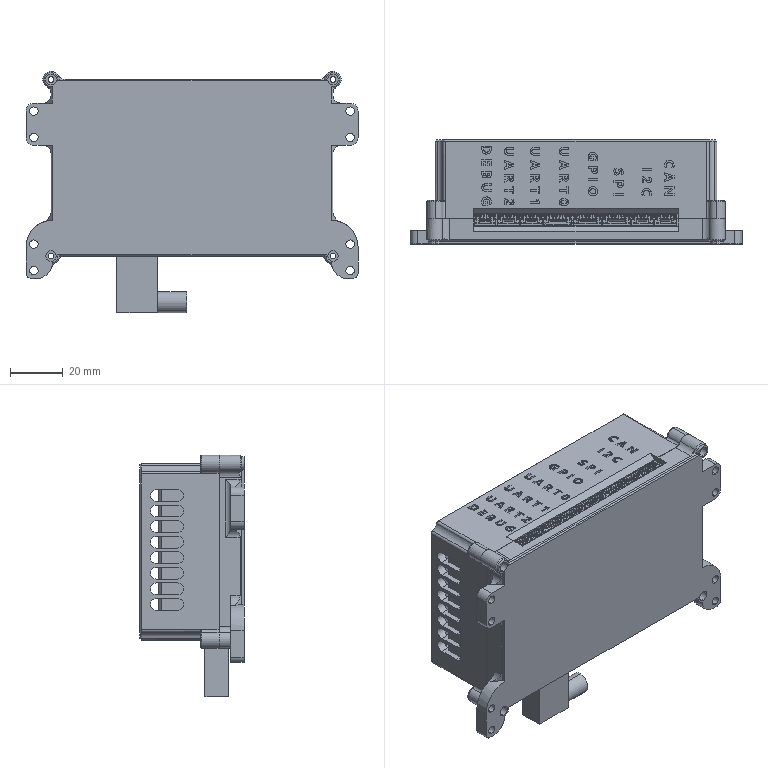Part | SolidWorks | 30 solids | 9467 faces | volume 99584 mm3 | plane 6902 | cylinder 1493 | spline 943 | cone 98 | torus 19 | sphere 12 | commonest cylinder face diameters 0.6 x202 0.3 x195 2 x128 0.2 x103 0.4 x81 4 x73